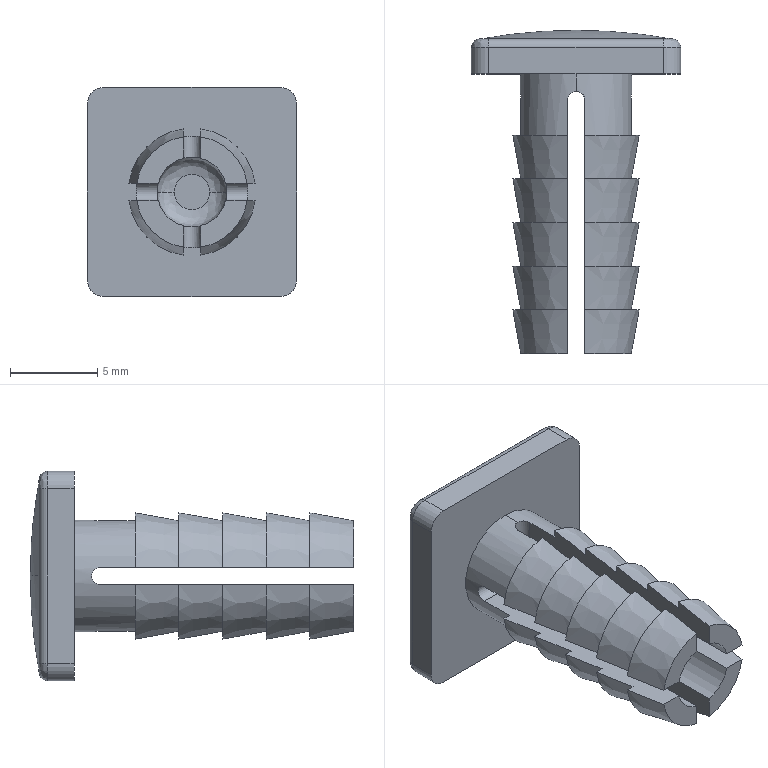Part | STEP file | 00369095_STOPFEN_BEFEST._IPM-AB-8-SW | 1 solid | 83 faces | box 12 x 18.5 x 12 mm | volume 599.689 mm3 | plane 39 | cone 20 | cylinder 16 | spline 8 | commonest cylinder face diameters 0.98 x4 1 x4 2 x4 4 x2 6.4 x2